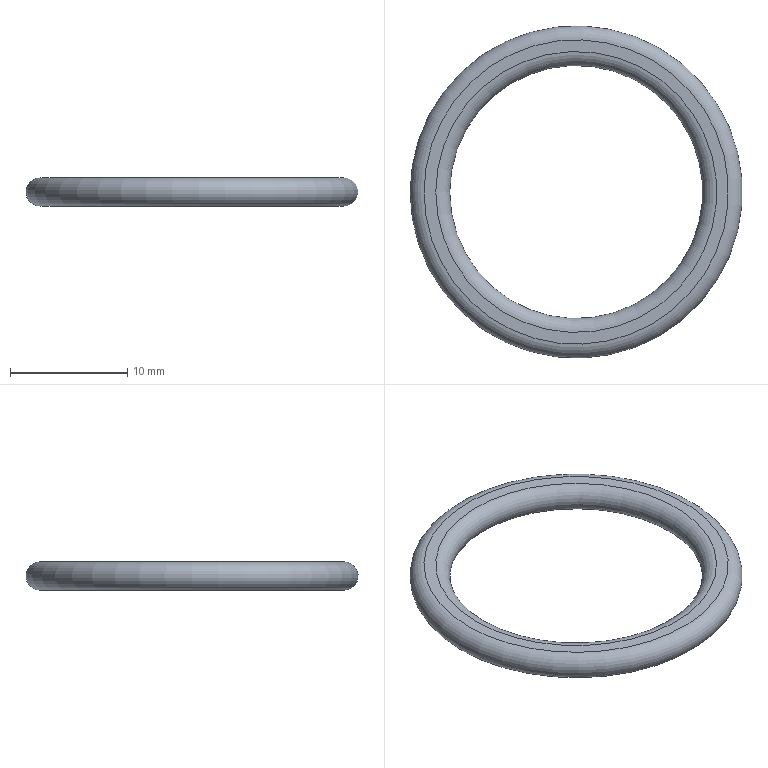Part | STEP file | solid 17 | 1 solid | 4 faces | box 28.401 x 28.401 x 2.4 mm | volume 543.953 mm3 | plane 2 | torus 2